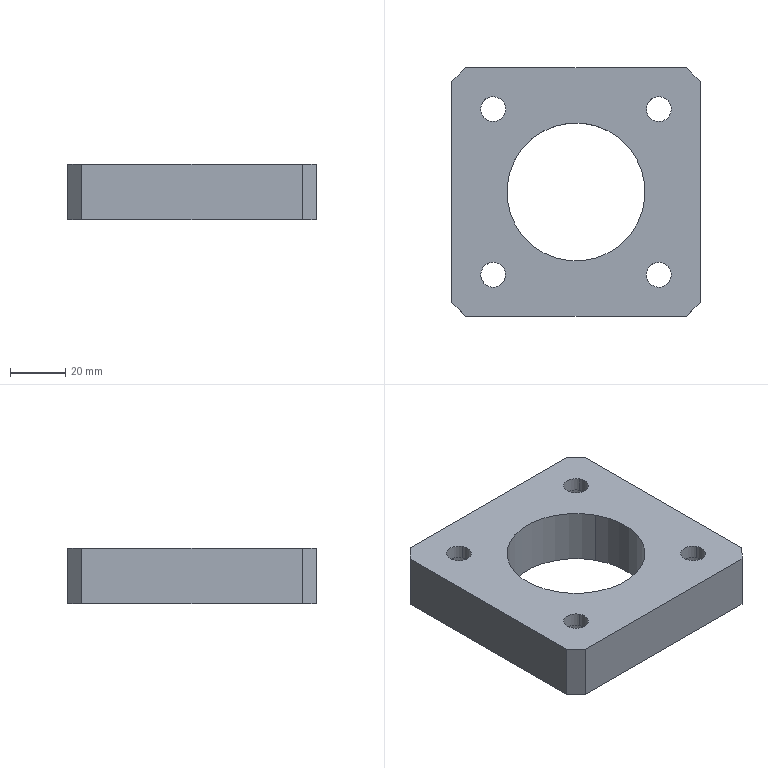Part | CATIA | 1 solid | 32 faces | box 90 x 90 x 20 mm | volume 109855 mm3 | cylinder 18 | plane 14 | commonest cylinder face diameters 9 x8 15 x8 50 x2
STEP:
#1=CARTESIAN_POINT('',(500.,-120.,-5.5));
#2=VERTEX_POINT('',#1);
#3=CARTESIAN_POINT('',(500.,-120.,14.5));
#4=VERTEX_POINT('',#3);
#5=CARTESIAN_POINT('',(500.,-120.,4.5));
#6=DIRECTION('',(0.,0.,-1.));
#7=VECTOR('',#6,1.);
#8=LINE('',#5,#7);
#9=EDGE_CURVE('',#2,#4,#8,.F.);
#10=ORIENTED_EDGE('',*,*,#9,.F.);
#11=CARTESIAN_POINT('',(495.,-125.,-5.5));
#12=VERTEX_POINT('',#11);
#13=CARTESIAN_POINT('',(497.5,-122.5,-5.5));
#14=DIRECTION('',(0.7071,0.7071,0.));
#15=VECTOR('',#14,1.);
#16=LINE('',#13,#15);
#17=EDGE_CURVE('',#2,#12,#16,.F.);
#18=ORIENTED_EDGE('',*,*,#17,.T.);
#19=CARTESIAN_POINT('',(495.,-125.,14.5));
#20=VERTEX_POINT('',#19);
#21=CARTESIAN_POINT('',(495.,-125.,4.5));
#22=DIRECTION('',(0.,0.,-1.));
#23=VECTOR('',#22,1.);
#24=LINE('',#21,#23);
#25=EDGE_CURVE('',#12,#20,#24,.F.);
#26=ORIENTED_EDGE('',*,*,#25,.T.);
#27=CARTESIAN_POINT('',(497.5,-122.5,14.5));
#28=DIRECTION('',(0.7071,0.7071,0.));
#29=VECTOR('',#28,1.);
#30=LINE('',#27,#29);
#31=EDGE_CURVE('',#20,#4,#30,.T.);
#32=ORIENTED_EDGE('',*,*,#31,.T.);
#33=EDGE_LOOP('',(#10,#18,#26,#32));
#34=FACE_OUTER_BOUND('',#33,.T.);
#35=CARTESIAN_POINT('',(495.,-125.,18.5));
#36=DIRECTION('',(0.7071,-0.7071,0.));
#37=DIRECTION('',(0.,0.,-1.));
#38=AXIS2_PLACEMENT_3D('',#35,#36,#37);
#39=PLANE('',#38);
#40=ADVANCED_FACE('',(#34),#39,.F.);
#41=CARTESIAN_POINT('',(495.,-205.,-5.5));
#42=VERTEX_POINT('',#41);
#43=CARTESIAN_POINT('',(495.,-205.,14.5));
#44=VERTEX_POINT('',#43);
#45=CARTESIAN_POINT('',(495.,-205.,4.5));
#46=DIRECTION('',(0.,0.,1.));
#47=VECTOR('',#46,1.);
#48=LINE('',#45,#47);
#49=EDGE_CURVE('',#42,#44,#48,.T.);
#50=ORIENTED_EDGE('',*,*,#49,.T.);
#51=CARTESIAN_POINT('',(495.,-165.,14.5));
#52=DIRECTION('',(0.,1.,0.));
#53=VECTOR('',#52,1.);
#54=LINE('',#51,#53);
#55=EDGE_CURVE('',#20,#44,#54,.F.);
#56=ORIENTED_EDGE('',*,*,#55,.F.);
#57=ORIENTED_EDGE('',*,*,#25,.F.);
#58=CARTESIAN_POINT('',(495.,-165.,-5.5));
#59=DIRECTION('',(0.,1.,0.));
#60=VECTOR('',#59,1.);
#61=LINE('',#58,#60);
#62=EDGE_CURVE('',#12,#42,#61,.F.);
#63=ORIENTED_EDGE('',*,*,#62,.T.);
#64=EDGE_LOOP('',(#50,#56,#57,#63));
#65=FACE_OUTER_BOUND('',#64,.T.);
#66=CARTESIAN_POINT('',(495.,-210.,-5.5));
#67=DIRECTION('',(1.,0.,0.));
#68=DIRECTION('',(0.,1.,0.));
#69=AXIS2_PLACEMENT_3D('',#66,#67,#68);
#70=PLANE('',#69);
#71=ADVANCED_FACE('',(#65),#70,.F.);
#72=ORIENTED_EDGE('',*,*,#49,.F.);
#73=CARTESIAN_POINT('',(500.,-210.,-5.5));
#74=VERTEX_POINT('',#73);
#75=CARTESIAN_POINT('',(497.5,-207.5,-5.5));
#76=DIRECTION('',(0.7071,-0.7071,0.));
#77=VECTOR('',#76,1.);
#78=LINE('',#75,#77);
#79=EDGE_CURVE('',#42,#74,#78,.T.);
#80=ORIENTED_EDGE('',*,*,#79,.T.);
#81=CARTESIAN_POINT('',(500.,-210.,14.5));
#82=VERTEX_POINT('',#81);
#83=CARTESIAN_POINT('',(500.,-210.,4.5));
#84=DIRECTION('',(0.,0.,1.));
#85=VECTOR('',#84,1.);
#86=LINE('',#83,#85);
#87=EDGE_CURVE('',#74,#82,#86,.T.);
#88=ORIENTED_EDGE('',*,*,#87,.T.);
#89=CARTESIAN_POINT('',(497.5,-207.5,14.5));
#90=DIRECTION('',(0.7071,-0.7071,0.));
#91=VECTOR('',#90,1.);
#92=LINE('',#89,#91);
#93=EDGE_CURVE('',#82,#44,#92,.F.);
#94=ORIENTED_EDGE('',*,*,#93,.T.);
#95=EDGE_LOOP('',(#72,#80,#88,#94));
#96=FACE_OUTER_BOUND('',#95,.T.);
#97=CARTESIAN_POINT('',(495.,-205.,-9.5));
#98=DIRECTION('',(0.7071,0.7071,0.));
#99=DIRECTION('',(0.,0.,1.));
#100=AXIS2_PLACEMENT_3D('',#97,#98,#99);
#101=PLANE('',#100);
#102=ADVANCED_FACE('',(#96),#101,.F.);
#103=CARTESIAN_POINT('',(580.,-210.,-5.5));
#104=VERTEX_POINT('',#103);
#105=CARTESIAN_POINT('',(580.,-210.,14.5));
#106=VERTEX_POINT('',#105);
#107=CARTESIAN_POINT('',(580.,-210.,4.5));
#108=DIRECTION('',(0.,0.,-1.));
#109=VECTOR('',#108,1.);
#110=LINE('',#107,#109);
#111=EDGE_CURVE('',#104,#106,#110,.F.);
#112=ORIENTED_EDGE('',*,*,#111,.T.);
#113=CARTESIAN_POINT('',(540.,-210.,14.5));
#114=DIRECTION('',(-1.,0.,0.));
#115=VECTOR('',#114,1.);
#116=LINE('',#113,#115);
#117=EDGE_CURVE('',#82,#106,#116,.F.);
#118=ORIENTED_EDGE('',*,*,#117,.F.);
#119=ORIENTED_EDGE('',*,*,#87,.F.);
#120=CARTESIAN_POINT('',(540.,-210.,-5.5));
#121=DIRECTION('',(-1.,0.,0.));
#122=VECTOR('',#121,1.);
#123=LINE('',#120,#122);
#124=EDGE_CURVE('',#74,#104,#123,.F.);
#125=ORIENTED_EDGE('',*,*,#124,.T.);
#126=EDGE_LOOP('',(#112,#118,#119,#125));
#127=FACE_OUTER_BOUND('',#126,.T.);
#128=CARTESIAN_POINT('',(585.,-210.,-5.5));
#129=DIRECTION('',(0.,1.,0.));
#130=DIRECTION('',(-1.,0.,0.));
#131=AXIS2_PLACEMENT_3D('',#128,#129,#130);
#132=PLANE('',#131);
#133=ADVANCED_FACE('',(#127),#132,.F.);
#134=ORIENTED_EDGE('',*,*,#111,.F.);
#135=CARTESIAN_POINT('',(585.,-205.,-5.5));
#136=VERTEX_POINT('',#135);
#137=CARTESIAN_POINT('',(582.5,-207.5,-5.5));
#138=DIRECTION('',(-0.7071,-0.7071,0.));
#139=VECTOR('',#138,1.);
#140=LINE('',#137,#139);
#141=EDGE_CURVE('',#104,#136,#140,.F.);
#142=ORIENTED_EDGE('',*,*,#141,.T.);
#143=CARTESIAN_POINT('',(585.,-205.,14.5));
#144=VERTEX_POINT('',#143);
#145=CARTESIAN_POINT('',(585.,-205.,4.5));
#146=DIRECTION('',(0.,0.,-1.));
#147=VECTOR('',#146,1.);
#148=LINE('',#145,#147);
#149=EDGE_CURVE('',#136,#144,#148,.F.);
#150=ORIENTED_EDGE('',*,*,#149,.T.);
#151=CARTESIAN_POINT('',(582.5,-207.5,14.5));
#152=DIRECTION('',(-0.7071,-0.7071,0.));
#153=VECTOR('',#152,1.);
#154=LINE('',#151,#153);
#155=EDGE_CURVE('',#144,#106,#154,.T.);
#156=ORIENTED_EDGE('',*,*,#155,.T.);
#157=EDGE_LOOP('',(#134,#142,#150,#156));
#158=FACE_OUTER_BOUND('',#157,.T.);
#159=CARTESIAN_POINT('',(585.,-205.,18.5));
#160=DIRECTION('',(-0.7071,0.7071,0.));
#161=DIRECTION('',(0.,0.,-1.));
#162=AXIS2_PLACEMENT_3D('',#159,#160,#161);
#163=PLANE('',#162);
#164=ADVANCED_FACE('',(#158),#163,.F.);
#165=CARTESIAN_POINT('',(580.,-120.,-5.5));
#166=VERTEX_POINT('',#165);
#167=CARTESIAN_POINT('',(580.,-120.,14.5));
#168=VERTEX_POINT('',#167);
#169=CARTESIAN_POINT('',(580.,-120.,4.5));
#170=DIRECTION('',(0.,0.,1.));
#171=VECTOR('',#170,1.);
#172=LINE('',#169,#171);
#173=EDGE_CURVE('',#166,#168,#172,.T.);
#174=ORIENTED_EDGE('',*,*,#173,.F.);
#175=CARTESIAN_POINT('',(540.,-120.,-5.5));
#176=DIRECTION('',(1.,0.,0.));
#177=VECTOR('',#176,1.);
#178=LINE('',#175,#177);
#179=EDGE_CURVE('',#166,#2,#178,.F.);
#180=ORIENTED_EDGE('',*,*,#179,.T.);
#181=ORIENTED_EDGE('',*,*,#9,.T.);
#182=CARTESIAN_POINT('',(540.,-120.,14.5));
#183=DIRECTION('',(1.,0.,0.));
#184=VECTOR('',#183,1.);
#185=LINE('',#182,#184);
#186=EDGE_CURVE('',#168,#4,#185,.F.);
#187=ORIENTED_EDGE('',*,*,#186,.F.);
#188=EDGE_LOOP('',(#174,#180,#181,#187));
#189=FACE_OUTER_BOUND('',#188,.T.);
#190=CARTESIAN_POINT('',(495.,-120.,-5.5));
#191=DIRECTION('',(0.,-1.,0.));
#192=DIRECTION('',(1.,0.,0.));
#193=AXIS2_PLACEMENT_3D('',#190,#191,#192);
#194=PLANE('',#193);
#195=ADVANCED_FACE('',(#189),#194,.F.);
#196=CARTESIAN_POINT('',(585.,-125.,-5.5));
#197=VERTEX_POINT('',#196);
#198=CARTESIAN_POINT('',(585.,-125.,14.5));
#199=VERTEX_POINT('',#198);
#200=CARTESIAN_POINT('',(585.,-125.,4.5));
#201=DIRECTION('',(0.,0.,1.));
#202=VECTOR('',#201,1.);
#203=LINE('',#200,#202);
#204=EDGE_CURVE('',#197,#199,#203,.T.);
#205=ORIENTED_EDGE('',*,*,#204,.T.);
#206=CARTESIAN_POINT('',(585.,-165.,14.5));
#207=DIRECTION('',(0.,-1.,0.));
#208=VECTOR('',#207,1.);
#209=LINE('',#206,#208);
#210=EDGE_CURVE('',#144,#199,#209,.F.);
#211=ORIENTED_EDGE('',*,*,#210,.F.);
#212=ORIENTED_EDGE('',*,*,#149,.F.);
#213=CARTESIAN_POINT('',(585.,-165.,-5.5));
#214=DIRECTION('',(0.,-1.,0.));
#215=VECTOR('',#214,1.);
#216=LINE('',#213,#215);
#217=EDGE_CURVE('',#136,#197,#216,.F.);
#218=ORIENTED_EDGE('',*,*,#217,.T.);
#219=EDGE_LOOP('',(#205,#211,#212,#218));
#220=FACE_OUTER_BOUND('',#219,.T.);
#221=CARTESIAN_POINT('',(585.,-120.,-5.5));
#222=DIRECTION('',(-1.,0.,0.));
#223=DIRECTION('',(0.,-1.,0.));
#224=AXIS2_PLACEMENT_3D('',#221,#222,#223);
#225=PLANE('',#224);
#226=ADVANCED_FACE('',(#220),#225,.F.);
#227=ORIENTED_EDGE('',*,*,#204,.F.);
#228=CARTESIAN_POINT('',(582.5,-122.5,-5.5));
#229=DIRECTION('',(-0.7071,0.7071,0.));
#230=VECTOR('',#229,1.);
#231=LINE('',#228,#230);
#232=EDGE_CURVE('',#197,#166,#231,.T.);
#233=ORIENTED_EDGE('',*,*,#232,.T.);
#234=ORIENTED_EDGE('',*,*,#173,.T.);
#235=CARTESIAN_POINT('',(582.5,-122.5,14.5));
#236=DIRECTION('',(-0.7071,0.7071,0.));
#237=VECTOR('',#236,1.);
#238=LINE('',#235,#237);
#239=EDGE_CURVE('',#168,#199,#238,.F.);
#240=ORIENTED_EDGE('',*,*,#239,.T.);
#241=EDGE_LOOP('',(#227,#233,#234,#240));
#242=FACE_OUTER_BOUND('',#241,.T.);
#243=CARTESIAN_POINT('',(585.,-125.,-9.5));
#244=DIRECTION('',(-0.7071,-0.7071,0.));
#245=DIRECTION('',(0.,0.,1.));
#246=AXIS2_PLACEMENT_3D('',#243,#244,#245);
#247=PLANE('',#246);
#248=ADVANCED_FACE('',(#242),#247,.F.);
#249=CARTESIAN_POINT('',(518.06,-176.986,14.5));
#250=VERTEX_POINT('',#249);
#251=CARTESIAN_POINT('',(561.94,-153.014,14.5));
#252=VERTEX_POINT('',#251);
#253=CARTESIAN_POINT('',(540.,-165.,14.5));
#254=DIRECTION('',(0.,0.,1.));
#255=AXIS2_PLACEMENT_3D('',#253,#254,$);
#256=CIRCLE('',#255,25.);
#257=EDGE_CURVE('',#250,#252,#256,.T.);
#258=ORIENTED_EDGE('',*,*,#257,.T.);
#259=CARTESIAN_POINT('',(561.94,-153.014,-5.5));
#260=VERTEX_POINT('',#259);
#261=CARTESIAN_POINT('',(561.94,-153.014,9.3));
#262=DIRECTION('',(0.,0.,1.));
#263=VECTOR('',#262,1.);
#264=LINE('',#261,#263);
#265=EDGE_CURVE('',#252,#260,#264,.F.);
#266=ORIENTED_EDGE('',*,*,#265,.T.);
#267=CARTESIAN_POINT('',(518.06,-176.986,-5.5));
#268=VERTEX_POINT('',#267);
#269=CARTESIAN_POINT('',(540.,-165.,-5.5));
#270=DIRECTION('',(0.,0.,1.));
#271=AXIS2_PLACEMENT_3D('',#269,#270,$);
#272=CIRCLE('',#271,25.);
#273=EDGE_CURVE('',#268,#260,#272,.T.);
#274=ORIENTED_EDGE('',*,*,#273,.F.);
#275=CARTESIAN_POINT('',(518.06,-176.986,9.3));
#276=DIRECTION('',(0.,0.,1.));
#277=VECTOR('',#276,1.);
#278=LINE('',#275,#277);
#279=EDGE_CURVE('',#250,#268,#278,.F.);
#280=ORIENTED_EDGE('',*,*,#279,.F.);
#281=EDGE_LOOP('',(#258,#266,#274,#280));
#282=FACE_OUTER_BOUND('',#281,.T.);
#283=CARTESIAN_POINT('',(540.,-165.,-5.4));
#284=DIRECTION('',(0.,0.,1.));
#285=DIRECTION('',(0.8776,0.4794,0.));
#286=AXIS2_PLACEMENT_3D('',#283,#284,#285);
#287=CYLINDRICAL_SURFACE('',#286,25.);
#288=ADVANCED_FACE('',(#282),#287,.F.);
#289=CARTESIAN_POINT('',(540.,-165.,14.5));
#290=DIRECTION('',(0.,0.,1.));
#291=AXIS2_PLACEMENT_3D('',#289,#290,$);
#292=CIRCLE('',#291,25.);
#293=EDGE_CURVE('',#252,#250,#292,.T.);
#294=ORIENTED_EDGE('',*,*,#293,.T.);
#295=ORIENTED_EDGE('',*,*,#279,.T.);
#296=CARTESIAN_POINT('',(540.,-165.,-5.5));
#297=DIRECTION('',(0.,0.,1.));
#298=AXIS2_PLACEMENT_3D('',#296,#297,$);
#299=CIRCLE('',#298,25.);
#300=EDGE_CURVE('',#260,#268,#299,.T.);
#301=ORIENTED_EDGE('',*,*,#300,.F.);
#302=ORIENTED_EDGE('',*,*,#265,.F.);
#303=EDGE_LOOP('',(#294,#295,#301,#302));
#304=FACE_OUTER_BOUND('',#303,.T.);
#305=ADVANCED_FACE('',(#304),#287,.F.);
#306=ORIENTED_EDGE('',*,*,#232,.F.);
#307=ORIENTED_EDGE('',*,*,#217,.F.);
#308=ORIENTED_EDGE('',*,*,#141,.F.);
#309=ORIENTED_EDGE('',*,*,#124,.F.);
#310=ORIENTED_EDGE('',*,*,#79,.F.);
#311=ORIENTED_EDGE('',*,*,#62,.F.);
#312=ORIENTED_EDGE('',*,*,#17,.F.);
#313=ORIENTED_EDGE('',*,*,#179,.F.);
#314=EDGE_LOOP('',(#306,#307,#308,#309,#310,#311,#312,#313));
#315=FACE_OUTER_BOUND('',#314,.T.);
#316=ORIENTED_EDGE('',*,*,#300,.T.);
#317=ORIENTED_EDGE('',*,*,#273,.T.);
#318=EDGE_LOOP('',(#316,#317));
#319=FACE_BOUND('',#318,.T.);
#320=CARTESIAN_POINT('',(576.582,-191.404,-5.5));
#321=VERTEX_POINT('',#320);
#322=CARTESIAN_POINT('',(563.418,-198.596,-5.5));
#323=VERTEX_POINT('',#322);
#324=CARTESIAN_POINT('',(570.,-195.,-5.5));
#325=DIRECTION('',(0.,0.,1.));
#326=AXIS2_PLACEMENT_3D('',#324,#325,$);
#327=CIRCLE('',#326,7.5);
#328=EDGE_CURVE('',#321,#323,#327,.T.);
#329=ORIENTED_EDGE('',*,*,#328,.T.);
#330=CARTESIAN_POINT('',(570.,-195.,-5.5));
#331=DIRECTION('',(0.,0.,1.));
#332=AXIS2_PLACEMENT_3D('',#330,#331,$);
#333=CIRCLE('',#332,7.5);
#334=EDGE_CURVE('',#323,#321,#333,.T.);
#335=ORIENTED_EDGE('',*,*,#334,.T.);
#336=EDGE_LOOP('',(#329,#335));
#337=FACE_BOUND('',#336,.T.);
#338=CARTESIAN_POINT('',(516.582,-191.404,-5.5));
#339=VERTEX_POINT('',#338);
#340=CARTESIAN_POINT('',(503.418,-198.596,-5.5));
#341=VERTEX_POINT('',#340);
#342=CARTESIAN_POINT('',(510.,-195.,-5.5));
#343=DIRECTION('',(0.,0.,1.));
#344=AXIS2_PLACEMENT_3D('',#342,#343,$);
#345=CIRCLE('',#344,7.5);
#346=EDGE_CURVE('',#339,#341,#345,.T.);
#347=ORIENTED_EDGE('',*,*,#346,.T.);
#348=CARTESIAN_POINT('',(510.,-195.,-5.5));
#349=DIRECTION('',(0.,0.,1.));
#350=AXIS2_PLACEMENT_3D('',#348,#349,$);
#351=CIRCLE('',#350,7.5);
#352=EDGE_CURVE('',#341,#339,#351,.T.);
#353=ORIENTED_EDGE('',*,*,#352,.T.);
#354=EDGE_LOOP('',(#347,#353));
#355=FACE_BOUND('',#354,.T.);
#356=CARTESIAN_POINT('',(576.582,-131.404,-5.5));
#357=VERTEX_POINT('',#356);
#358=CARTESIAN_POINT('',(563.418,-138.596,-5.5));
#359=VERTEX_POINT('',#358);
#360=CARTESIAN_POINT('',(570.,-135.,-5.5));
#361=DIRECTION('',(0.,0.,1.));
#362=AXIS2_PLACEMENT_3D('',#360,#361,$);
#363=CIRCLE('',#362,7.5);
#364=EDGE_CURVE('',#357,#359,#363,.T.);
#365=ORIENTED_EDGE('',*,*,#364,.T.);
#366=CARTESIAN_POINT('',(570.,-135.,-5.5));
#367=DIRECTION('',(0.,0.,1.));
#368=AXIS2_PLACEMENT_3D('',#366,#367,$);
#369=CIRCLE('',#368,7.5);
#370=EDGE_CURVE('',#359,#357,#369,.T.);
#371=ORIENTED_EDGE('',*,*,#370,.T.);
#372=EDGE_LOOP('',(#365,#371));
#373=FACE_BOUND('',#372,.T.);
#374=CARTESIAN_POINT('',(516.582,-131.404,-5.5));
#375=VERTEX_POINT('',#374);
#376=CARTESIAN_POINT('',(503.418,-138.596,-5.5));
#377=VERTEX_POINT('',#376);
#378=CARTESIAN_POINT('',(510.,-135.,-5.5));
#379=DIRECTION('',(0.,0.,1.));
#380=AXIS2_PLACEMENT_3D('',#378,#379,$);
#381=CIRCLE('',#380,7.5);
#382=EDGE_CURVE('',#375,#377,#381,.T.);
#383=ORIENTED_EDGE('',*,*,#382,.T.);
#384=CARTESIAN_POINT('',(510.,-135.,-5.5));
#385=DIRECTION('',(0.,0.,1.));
#386=AXIS2_PLACEMENT_3D('',#384,#385,$);
#387=CIRCLE('',#386,7.5);
#388=EDGE_CURVE('',#377,#375,#387,.T.);
#389=ORIENTED_EDGE('',*,*,#388,.T.);
#390=EDGE_LOOP('',(#383,#389));
#391=FACE_BOUND('',#390,.T.);
#392=CARTESIAN_POINT('',(0.,0.,-5.5));
#393=DIRECTION('',(0.,0.,1.));
#394=DIRECTION('',(1.,0.,0.));
#395=AXIS2_PLACEMENT_3D('',#392,#393,#394);
#396=PLANE('',#395);
#397=ADVANCED_FACE('',(#315,#319,#337,#355,#373,#391),#396,.F.);
#398=ORIENTED_EDGE('',*,*,#186,.T.);
#399=ORIENTED_EDGE('',*,*,#31,.F.);
#400=ORIENTED_EDGE('',*,*,#55,.T.);
#401=ORIENTED_EDGE('',*,*,#93,.F.);
#402=ORIENTED_EDGE('',*,*,#117,.T.);
#403=ORIENTED_EDGE('',*,*,#155,.F.);
#404=ORIENTED_EDGE('',*,*,#210,.T.);
#405=ORIENTED_EDGE('',*,*,#239,.F.);
#406=EDGE_LOOP('',(#398,#399,#400,#401,#402,#403,#404,#405));
#407=FACE_OUTER_BOUND('',#406,.T.);
#408=ORIENTED_EDGE('',*,*,#293,.F.);
#409=ORIENTED_EDGE('',*,*,#257,.F.);
#410=EDGE_LOOP('',(#408,#409));
#411=FACE_BOUND('',#410,.T.);
#412=CARTESIAN_POINT('',(566.051,-197.157,14.5));
#413=VERTEX_POINT('',#412);
#414=CARTESIAN_POINT('',(573.949,-192.843,14.5));
#415=VERTEX_POINT('',#414);
#416=CARTESIAN_POINT('',(570.,-195.,14.5));
#417=DIRECTION('',(0.,0.,1.));
#418=AXIS2_PLACEMENT_3D('',#416,#417,$);
#419=CIRCLE('',#418,4.5);
#420=EDGE_CURVE('',#413,#415,#419,.T.);
#421=ORIENTED_EDGE('',*,*,#420,.F.);
#422=CARTESIAN_POINT('',(570.,-195.,14.5));
#423=DIRECTION('',(0.,0.,1.));
#424=AXIS2_PLACEMENT_3D('',#422,#423,$);
#425=CIRCLE('',#424,4.5);
#426=EDGE_CURVE('',#415,#413,#425,.T.);
#427=ORIENTED_EDGE('',*,*,#426,.F.);
#428=EDGE_LOOP('',(#421,#427));
#429=FACE_BOUND('',#428,.T.);
#430=CARTESIAN_POINT('',(506.051,-197.157,14.5));
#431=VERTEX_POINT('',#430);
#432=CARTESIAN_POINT('',(513.949,-192.843,14.5));
#433=VERTEX_POINT('',#432);
#434=CARTESIAN_POINT('',(510.,-195.,14.5));
#435=DIRECTION('',(0.,0.,1.));
#436=AXIS2_PLACEMENT_3D('',#434,#435,$);
#437=CIRCLE('',#436,4.5);
#438=EDGE_CURVE('',#431,#433,#437,.T.);
#439=ORIENTED_EDGE('',*,*,#438,.F.);
#440=CARTESIAN_POINT('',(510.,-195.,14.5));
#441=DIRECTION('',(0.,0.,1.));
#442=AXIS2_PLACEMENT_3D('',#440,#441,$);
#443=CIRCLE('',#442,4.5);
#444=EDGE_CURVE('',#433,#431,#443,.T.);
#445=ORIENTED_EDGE('',*,*,#444,.F.);
#446=EDGE_LOOP('',(#439,#445));
#447=FACE_BOUND('',#446,.T.);
#448=CARTESIAN_POINT('',(566.051,-137.157,14.5));
#449=VERTEX_POINT('',#448);
#450=CARTESIAN_POINT('',(573.949,-132.843,14.5));
#451=VERTEX_POINT('',#450);
#452=CARTESIAN_POINT('',(570.,-135.,14.5));
#453=DIRECTION('',(0.,0.,1.));
#454=AXIS2_PLACEMENT_3D('',#452,#453,$);
#455=CIRCLE('',#454,4.5);
#456=EDGE_CURVE('',#449,#451,#455,.T.);
#457=ORIENTED_EDGE('',*,*,#456,.F.);
#458=CARTESIAN_POINT('',(570.,-135.,14.5));
#459=DIRECTION('',(0.,0.,1.));
#460=AXIS2_PLACEMENT_3D('',#458,#459,$);
#461=CIRCLE('',#460,4.5);
#462=EDGE_CURVE('',#451,#449,#461,.T.);
#463=ORIENTED_EDGE('',*,*,#462,.F.);
#464=EDGE_LOOP('',(#457,#463));
#465=FACE_BOUND('',#464,.T.);
#466=CARTESIAN_POINT('',(506.051,-137.157,14.5));
#467=VERTEX_POINT('',#466);
#468=CARTESIAN_POINT('',(513.949,-132.843,14.5));
#469=VERTEX_POINT('',#468);
#470=CARTESIAN_POINT('',(510.,-135.,14.5));
#471=DIRECTION('',(0.,0.,1.));
#472=AXIS2_PLACEMENT_3D('',#470,#471,$);
#473=CIRCLE('',#472,4.5);
#474=EDGE_CURVE('',#467,#469,#473,.T.);
#475=ORIENTED_EDGE('',*,*,#474,.F.);
#476=CARTESIAN_POINT('',(510.,-135.,14.5));
#477=DIRECTION('',(0.,0.,1.));
#478=AXIS2_PLACEMENT_3D('',#476,#477,$);
#479=CIRCLE('',#478,4.5);
#480=EDGE_CURVE('',#469,#467,#479,.T.);
#481=ORIENTED_EDGE('',*,*,#480,.F.);
#482=EDGE_LOOP('',(#475,#481));
#483=FACE_BOUND('',#482,.T.);
#484=CARTESIAN_POINT('',(0.,0.,14.5));
#485=DIRECTION('',(0.,0.,1.));
#486=DIRECTION('',(1.,0.,0.));
#487=AXIS2_PLACEMENT_3D('',#484,#485,#486);
#488=PLANE('',#487);
#489=ADVANCED_FACE('',(#407,#411,#429,#447,#465,#483),#488,.T.);
#490=CARTESIAN_POINT('',(576.582,-131.404,9.5));
#491=VERTEX_POINT('',#490);
#492=CARTESIAN_POINT('',(563.418,-138.596,9.5));
#493=VERTEX_POINT('',#492);
#494=CARTESIAN_POINT('',(570.,-135.,9.5));
#495=DIRECTION('',(0.,0.,1.));
#496=AXIS2_PLACEMENT_3D('',#494,#495,$);
#497=CIRCLE('',#496,7.5);
#498=EDGE_CURVE('',#491,#493,#497,.T.);
#499=ORIENTED_EDGE('',*,*,#498,.F.);
#500=CARTESIAN_POINT('',(570.,-135.,9.5));
#501=DIRECTION('',(0.,0.,1.));
#502=AXIS2_PLACEMENT_3D('',#500,#501,$);
#503=CIRCLE('',#502,7.5);
#504=EDGE_CURVE('',#493,#491,#503,.T.);
#505=ORIENTED_EDGE('',*,*,#504,.F.);
#506=EDGE_LOOP('',(#499,#505));
#507=FACE_OUTER_BOUND('',#506,.T.);
#508=CARTESIAN_POINT('',(566.051,-137.157,9.5));
#509=VERTEX_POINT('',#508);
#510=CARTESIAN_POINT('',(573.949,-132.843,9.5));
#511=VERTEX_POINT('',#510);
#512=CARTESIAN_POINT('',(570.,-135.,9.5));
#513=DIRECTION('',(0.,0.,1.));
#514=AXIS2_PLACEMENT_3D('',#512,#513,$);
#515=CIRCLE('',#514,4.5);
#516=EDGE_CURVE('',#509,#511,#515,.T.);
#517=ORIENTED_EDGE('',*,*,#516,.T.);
#518=CARTESIAN_POINT('',(570.,-135.,9.5));
#519=DIRECTION('',(0.,0.,1.));
#520=AXIS2_PLACEMENT_3D('',#518,#519,$);
#521=CIRCLE('',#520,4.5);
#522=EDGE_CURVE('',#511,#509,#521,.T.);
#523=ORIENTED_EDGE('',*,*,#522,.T.);
#524=EDGE_LOOP('',(#517,#523));
#525=FACE_BOUND('',#524,.T.);
#526=CARTESIAN_POINT('',(574.5,-195.,9.5));
#527=DIRECTION('',(0.,0.,1.));
#528=DIRECTION('',(1.,0.,0.));
#529=AXIS2_PLACEMENT_3D('',#526,#527,#528);
#530=PLANE('',#529);
#531=ADVANCED_FACE('',(#507,#525),#530,.F.);
#532=ORIENTED_EDGE('',*,*,#370,.F.);
#533=CARTESIAN_POINT('',(563.418,-138.596,1.8));
#534=DIRECTION('',(0.,0.,1.));
#535=VECTOR('',#534,1.);
#536=LINE('',#533,#535);
#537=EDGE_CURVE('',#493,#359,#536,.F.);
#538=ORIENTED_EDGE('',*,*,#537,.F.);
#539=ORIENTED_EDGE('',*,*,#504,.T.);
#540=CARTESIAN_POINT('',(576.582,-131.404,1.8));
#541=DIRECTION('',(0.,0.,1.));
#542=VECTOR('',#541,1.);
#543=LINE('',#540,#542);
#544=EDGE_CURVE('',#491,#357,#543,.F.);
#545=ORIENTED_EDGE('',*,*,#544,.T.);
#546=EDGE_LOOP('',(#532,#538,#539,#545));
#547=FACE_OUTER_BOUND('',#546,.T.);
#548=CARTESIAN_POINT('',(570.,-135.,-5.4));
#549=DIRECTION('',(0.,0.,1.));
#550=DIRECTION('',(0.8776,0.4794,0.));
#551=AXIS2_PLACEMENT_3D('',#548,#549,#550);
#552=CYLINDRICAL_SURFACE('',#551,7.5);
#553=ADVANCED_FACE('',(#547),#552,.F.);
#554=ORIENTED_EDGE('',*,*,#364,.F.);
#555=ORIENTED_EDGE('',*,*,#544,.F.);
#556=ORIENTED_EDGE('',*,*,#498,.T.);
#557=ORIENTED_EDGE('',*,*,#537,.T.);
#558=EDGE_LOOP('',(#554,#555,#556,#557));
#559=FACE_OUTER_BOUND('',#558,.T.);
#560=ADVANCED_FACE('',(#559),#552,.F.);
#561=ORIENTED_EDGE('',*,*,#462,.T.);
#562=CARTESIAN_POINT('',(566.051,-137.157,12.2));
#563=DIRECTION('',(0.,0.,1.));
#564=VECTOR('',#563,1.);
#565=LINE('',#562,#564);
#566=EDGE_CURVE('',#449,#509,#565,.F.);
#567=ORIENTED_EDGE('',*,*,#566,.T.);
#568=ORIENTED_EDGE('',*,*,#522,.F.);
#569=CARTESIAN_POINT('',(573.949,-132.843,12.2));
#570=DIRECTION('',(0.,0.,1.));
#571=VECTOR('',#570,1.);
#572=LINE('',#569,#571);
#573=EDGE_CURVE('',#451,#511,#572,.F.);
#574=ORIENTED_EDGE('',*,*,#573,.F.);
#575=EDGE_LOOP('',(#561,#567,#568,#574));
#576=FACE_OUTER_BOUND('',#575,.T.);
#577=CARTESIAN_POINT('',(570.,-135.,-5.4));
#578=DIRECTION('',(0.,0.,1.));
#579=DIRECTION('',(0.8776,0.4794,0.));
#580=AXIS2_PLACEMENT_3D('',#577,#578,#579);
#581=CYLINDRICAL_SURFACE('',#580,4.5);
#582=ADVANCED_FACE('',(#576),#581,.F.);
#583=ORIENTED_EDGE('',*,*,#456,.T.);
#584=ORIENTED_EDGE('',*,*,#573,.T.);
#585=ORIENTED_EDGE('',*,*,#516,.F.);
#586=ORIENTED_EDGE('',*,*,#566,.F.);
#587=EDGE_LOOP('',(#583,#584,#585,#586));
#588=FACE_OUTER_BOUND('',#587,.T.);
#589=ADVANCED_FACE('',(#588),#581,.F.);
#590=CARTESIAN_POINT('',(516.582,-191.404,9.5));
#591=VERTEX_POINT('',#590);
#592=CARTESIAN_POINT('',(503.418,-198.596,9.5));
#593=VERTEX_POINT('',#592);
#594=CARTESIAN_POINT('',(510.,-195.,9.5));
#595=DIRECTION('',(0.,0.,1.));
#596=AXIS2_PLACEMENT_3D('',#594,#595,$);
#597=CIRCLE('',#596,7.5);
#598=EDGE_CURVE('',#591,#593,#597,.T.);
#599=ORIENTED_EDGE('',*,*,#598,.F.);
#600=CARTESIAN_POINT('',(510.,-195.,9.5));
#601=DIRECTION('',(0.,0.,1.));
#602=AXIS2_PLACEMENT_3D('',#600,#601,$);
#603=CIRCLE('',#602,7.5);
#604=EDGE_CURVE('',#593,#591,#603,.T.);
#605=ORIENTED_EDGE('',*,*,#604,.F.);
#606=EDGE_LOOP('',(#599,#605));
#607=FACE_OUTER_BOUND('',#606,.T.);
#608=CARTESIAN_POINT('',(506.051,-197.157,9.5));
#609=VERTEX_POINT('',#608);
#610=CARTESIAN_POINT('',(513.949,-192.843,9.5));
#611=VERTEX_POINT('',#610);
#612=CARTESIAN_POINT('',(510.,-195.,9.5));
#613=DIRECTION('',(0.,0.,1.));
#614=AXIS2_PLACEMENT_3D('',#612,#613,$);
#615=CIRCLE('',#614,4.5);
#616=EDGE_CURVE('',#609,#611,#615,.T.);
#617=ORIENTED_EDGE('',*,*,#616,.T.);
#618=CARTESIAN_POINT('',(510.,-195.,9.5));
#619=DIRECTION('',(0.,0.,1.));
#620=AXIS2_PLACEMENT_3D('',#618,#619,$);
#621=CIRCLE('',#620,4.5);
#622=EDGE_CURVE('',#611,#609,#621,.T.);
#623=ORIENTED_EDGE('',*,*,#622,.T.);
#624=EDGE_LOOP('',(#617,#623));
#625=FACE_BOUND('',#624,.T.);
#626=ADVANCED_FACE('',(#607,#625),#530,.F.);
#627=ORIENTED_EDGE('',*,*,#352,.F.);
#628=CARTESIAN_POINT('',(503.418,-198.596,1.8));
#629=DIRECTION('',(0.,0.,1.));
#630=VECTOR('',#629,1.);
#631=LINE('',#628,#630);
#632=EDGE_CURVE('',#593,#341,#631,.F.);
#633=ORIENTED_EDGE('',*,*,#632,.F.);
#634=ORIENTED_EDGE('',*,*,#604,.T.);
#635=CARTESIAN_POINT('',(516.582,-191.404,1.8));
#636=DIRECTION('',(0.,0.,1.));
#637=VECTOR('',#636,1.);
#638=LINE('',#635,#637);
#639=EDGE_CURVE('',#591,#339,#638,.F.);
#640=ORIENTED_EDGE('',*,*,#639,.T.);
#641=EDGE_LOOP('',(#627,#633,#634,#640));
#642=FACE_OUTER_BOUND('',#641,.T.);
#643=CARTESIAN_POINT('',(510.,-195.,-5.4));
#644=DIRECTION('',(0.,0.,1.));
#645=DIRECTION('',(0.8776,0.4794,0.));
#646=AXIS2_PLACEMENT_3D('',#643,#644,#645);
#647=CYLINDRICAL_SURFACE('',#646,7.5);
#648=ADVANCED_FACE('',(#642),#647,.F.);
#649=ORIENTED_EDGE('',*,*,#346,.F.);
#650=ORIENTED_EDGE('',*,*,#639,.F.);
#651=ORIENTED_EDGE('',*,*,#598,.T.);
#652=ORIENTED_EDGE('',*,*,#632,.T.);
#653=EDGE_LOOP('',(#649,#650,#651,#652));
#654=FACE_OUTER_BOUND('',#653,.T.);
#655=ADVANCED_FACE('',(#654),#647,.F.);
#656=ORIENTED_EDGE('',*,*,#444,.T.);
#657=CARTESIAN_POINT('',(506.051,-197.157,12.2));
#658=DIRECTION('',(0.,0.,1.));
#659=VECTOR('',#658,1.);
#660=LINE('',#657,#659);
#661=EDGE_CURVE('',#431,#609,#660,.F.);
#662=ORIENTED_EDGE('',*,*,#661,.T.);
#663=ORIENTED_EDGE('',*,*,#622,.F.);
#664=CARTESIAN_POINT('',(513.949,-192.843,12.2));
#665=DIRECTION('',(0.,0.,1.));
#666=VECTOR('',#665,1.);
#667=LINE('',#664,#666);
#668=EDGE_CURVE('',#433,#611,#667,.F.);
#669=ORIENTED_EDGE('',*,*,#668,.F.);
#670=EDGE_LOOP('',(#656,#662,#663,#669));
#671=FACE_OUTER_BOUND('',#670,.T.);
#672=CARTESIAN_POINT('',(510.,-195.,-5.4));
#673=DIRECTION('',(0.,0.,1.));
#674=DIRECTION('',(0.8776,0.4794,0.));
#675=AXIS2_PLACEMENT_3D('',#672,#673,#674);
#676=CYLINDRICAL_SURFACE('',#675,4.5);
#677=ADVANCED_FACE('',(#671),#676,.F.);
#678=ORIENTED_EDGE('',*,*,#438,.T.);
#679=ORIENTED_EDGE('',*,*,#668,.T.);
#680=ORIENTED_EDGE('',*,*,#616,.F.);
#681=ORIENTED_EDGE('',*,*,#661,.F.);
#682=EDGE_LOOP('',(#678,#679,#680,#681));
#683=FACE_OUTER_BOUND('',#682,.T.);
#684=ADVANCED_FACE('',(#683),#676,.F.);
#685=CARTESIAN_POINT('',(516.582,-131.404,9.5));
#686=VERTEX_POINT('',#685);
#687=CARTESIAN_POINT('',(503.418,-138.596,9.5));
#688=VERTEX_POINT('',#687);
#689=CARTESIAN_POINT('',(510.,-135.,9.5));
#690=DIRECTION('',(0.,0.,1.));
#691=AXIS2_PLACEMENT_3D('',#689,#690,$);
#692=CIRCLE('',#691,7.5);
#693=EDGE_CURVE('',#686,#688,#692,.T.);
#694=ORIENTED_EDGE('',*,*,#693,.F.);
#695=CARTESIAN_POINT('',(510.,-135.,9.5));
#696=DIRECTION('',(0.,0.,1.));
#697=AXIS2_PLACEMENT_3D('',#695,#696,$);
#698=CIRCLE('',#697,7.5);
#699=EDGE_CURVE('',#688,#686,#698,.T.);
#700=ORIENTED_EDGE('',*,*,#699,.F.);
#701=EDGE_LOOP('',(#694,#700));
#702=FACE_OUTER_BOUND('',#701,.T.);
#703=CARTESIAN_POINT('',(506.051,-137.157,9.5));
#704=VERTEX_POINT('',#703);
#705=CARTESIAN_POINT('',(513.949,-132.843,9.5));
#706=VERTEX_POINT('',#705);
#707=CARTESIAN_POINT('',(510.,-135.,9.5));
#708=DIRECTION('',(0.,0.,1.));
#709=AXIS2_PLACEMENT_3D('',#707,#708,$);
#710=CIRCLE('',#709,4.5);
#711=EDGE_CURVE('',#704,#706,#710,.T.);
#712=ORIENTED_EDGE('',*,*,#711,.T.);
#713=CARTESIAN_POINT('',(510.,-135.,9.5));
#714=DIRECTION('',(0.,0.,1.));
#715=AXIS2_PLACEMENT_3D('',#713,#714,$);
#716=CIRCLE('',#715,4.5);
#717=EDGE_CURVE('',#706,#704,#716,.T.);
#718=ORIENTED_EDGE('',*,*,#717,.T.);
#719=EDGE_LOOP('',(#712,#718));
#720=FACE_BOUND('',#719,.T.);
#721=ADVANCED_FACE('',(#702,#720),#530,.F.);
#722=ORIENTED_EDGE('',*,*,#388,.F.);
#723=CARTESIAN_POINT('',(503.418,-138.596,1.8));
#724=DIRECTION('',(0.,0.,1.));
#725=VECTOR('',#724,1.);
#726=LINE('',#723,#725);
#727=EDGE_CURVE('',#688,#377,#726,.F.);
#728=ORIENTED_EDGE('',*,*,#727,.F.);
#729=ORIENTED_EDGE('',*,*,#699,.T.);
#730=CARTESIAN_POINT('',(516.582,-131.404,1.8));
#731=DIRECTION('',(0.,0.,1.));
#732=VECTOR('',#731,1.);
#733=LINE('',#730,#732);
#734=EDGE_CURVE('',#686,#375,#733,.F.);
#735=ORIENTED_EDGE('',*,*,#734,.T.);
#736=EDGE_LOOP('',(#722,#728,#729,#735));
#737=FACE_OUTER_BOUND('',#736,.T.);
#738=CARTESIAN_POINT('',(510.,-135.,-5.4));
#739=DIRECTION('',(0.,0.,1.));
#740=DIRECTION('',(0.8776,0.4794,0.));
#741=AXIS2_PLACEMENT_3D('',#738,#739,#740);
#742=CYLINDRICAL_SURFACE('',#741,7.5);
#743=ADVANCED_FACE('',(#737),#742,.F.);
#744=ORIENTED_EDGE('',*,*,#382,.F.);
#745=ORIENTED_EDGE('',*,*,#734,.F.);
#746=ORIENTED_EDGE('',*,*,#693,.T.);
#747=ORIENTED_EDGE('',*,*,#727,.T.);
#748=EDGE_LOOP('',(#744,#745,#746,#747));
#749=FACE_OUTER_BOUND('',#748,.T.);
#750=ADVANCED_FACE('',(#749),#742,.F.);
#751=ORIENTED_EDGE('',*,*,#480,.T.);
#752=CARTESIAN_POINT('',(506.051,-137.157,12.2));
#753=DIRECTION('',(0.,0.,1.));
#754=VECTOR('',#753,1.);
#755=LINE('',#752,#754);
#756=EDGE_CURVE('',#467,#704,#755,.F.);
#757=ORIENTED_EDGE('',*,*,#756,.T.);
#758=ORIENTED_EDGE('',*,*,#717,.F.);
#759=CARTESIAN_POINT('',(513.949,-132.843,12.2));
#760=DIRECTION('',(0.,0.,1.));
#761=VECTOR('',#760,1.);
#762=LINE('',#759,#761);
#763=EDGE_CURVE('',#469,#706,#762,.F.);
#764=ORIENTED_EDGE('',*,*,#763,.F.);
#765=EDGE_LOOP('',(#751,#757,#758,#764));
#766=FACE_OUTER_BOUND('',#765,.T.);
#767=CARTESIAN_POINT('',(510.,-135.,-5.4));
#768=DIRECTION('',(0.,0.,1.));
#769=DIRECTION('',(0.8776,0.4794,0.));
#770=AXIS2_PLACEMENT_3D('',#767,#768,#769);
#771=CYLINDRICAL_SURFACE('',#770,4.5);
#772=ADVANCED_FACE('',(#766),#771,.F.);
#773=ORIENTED_EDGE('',*,*,#474,.T.);
#774=ORIENTED_EDGE('',*,*,#763,.T.);
#775=ORIENTED_EDGE('',*,*,#711,.F.);
#776=ORIENTED_EDGE('',*,*,#756,.F.);
#777=EDGE_LOOP('',(#773,#774,#775,#776));
#778=FACE_OUTER_BOUND('',#777,.T.);
#779=ADVANCED_FACE('',(#778),#771,.F.);
#780=CARTESIAN_POINT('',(576.582,-191.404,9.5));
#781=VERTEX_POINT('',#780);
#782=CARTESIAN_POINT('',(563.418,-198.596,9.5));
#783=VERTEX_POINT('',#782);
#784=CARTESIAN_POINT('',(570.,-195.,9.5));
#785=DIRECTION('',(0.,0.,1.));
#786=AXIS2_PLACEMENT_3D('',#784,#785,$);
#787=CIRCLE('',#786,7.5);
#788=EDGE_CURVE('',#781,#783,#787,.T.);
#789=ORIENTED_EDGE('',*,*,#788,.F.);
#790=CARTESIAN_POINT('',(570.,-195.,9.5));
#791=DIRECTION('',(0.,0.,1.));
#792=AXIS2_PLACEMENT_3D('',#790,#791,$);
#793=CIRCLE('',#792,7.5);
#794=EDGE_CURVE('',#783,#781,#793,.T.);
#795=ORIENTED_EDGE('',*,*,#794,.F.);
#796=EDGE_LOOP('',(#789,#795));
#797=FACE_OUTER_BOUND('',#796,.T.);
#798=CARTESIAN_POINT('',(566.051,-197.157,9.5));
#799=VERTEX_POINT('',#798);
#800=CARTESIAN_POINT('',(573.949,-192.843,9.5));
#801=VERTEX_POINT('',#800);
#802=CARTESIAN_POINT('',(570.,-195.,9.5));
#803=DIRECTION('',(0.,0.,1.));
#804=AXIS2_PLACEMENT_3D('',#802,#803,$);
#805=CIRCLE('',#804,4.5);
#806=EDGE_CURVE('',#799,#801,#805,.T.);
#807=ORIENTED_EDGE('',*,*,#806,.T.);
#808=CARTESIAN_POINT('',(570.,-195.,9.5));
#809=DIRECTION('',(0.,0.,1.));
#810=AXIS2_PLACEMENT_3D('',#808,#809,$);
#811=CIRCLE('',#810,4.5);
#812=EDGE_CURVE('',#801,#799,#811,.T.);
#813=ORIENTED_EDGE('',*,*,#812,.T.);
#814=EDGE_LOOP('',(#807,#813));
#815=FACE_BOUND('',#814,.T.);
#816=ADVANCED_FACE('',(#797,#815),#530,.F.);
#817=ORIENTED_EDGE('',*,*,#334,.F.);
#818=CARTESIAN_POINT('',(563.418,-198.596,1.8));
#819=DIRECTION('',(0.,0.,1.));
#820=VECTOR('',#819,1.);
#821=LINE('',#818,#820);
#822=EDGE_CURVE('',#783,#323,#821,.F.);
#823=ORIENTED_EDGE('',*,*,#822,.F.);
#824=ORIENTED_EDGE('',*,*,#794,.T.);
#825=CARTESIAN_POINT('',(576.582,-191.404,1.8));
#826=DIRECTION('',(0.,0.,1.));
#827=VECTOR('',#826,1.);
#828=LINE('',#825,#827);
#829=EDGE_CURVE('',#781,#321,#828,.F.);
#830=ORIENTED_EDGE('',*,*,#829,.T.);
#831=EDGE_LOOP('',(#817,#823,#824,#830));
#832=FACE_OUTER_BOUND('',#831,.T.);
#833=CARTESIAN_POINT('',(570.,-195.,-5.4));
#834=DIRECTION('',(0.,0.,1.));
#835=DIRECTION('',(0.8776,0.4794,0.));
#836=AXIS2_PLACEMENT_3D('',#833,#834,#835);
#837=CYLINDRICAL_SURFACE('',#836,7.5);
#838=ADVANCED_FACE('',(#832),#837,.F.);
#839=ORIENTED_EDGE('',*,*,#328,.F.);
#840=ORIENTED_EDGE('',*,*,#829,.F.);
#841=ORIENTED_EDGE('',*,*,#788,.T.);
#842=ORIENTED_EDGE('',*,*,#822,.T.);
#843=EDGE_LOOP('',(#839,#840,#841,#842));
#844=FACE_OUTER_BOUND('',#843,.T.);
#845=ADVANCED_FACE('',(#844),#837,.F.);
#846=ORIENTED_EDGE('',*,*,#426,.T.);
#847=CARTESIAN_POINT('',(566.051,-197.157,12.2));
#848=DIRECTION('',(0.,0.,1.));
#849=VECTOR('',#848,1.);
#850=LINE('',#847,#849);
#851=EDGE_CURVE('',#413,#799,#850,.F.);
#852=ORIENTED_EDGE('',*,*,#851,.T.);
#853=ORIENTED_EDGE('',*,*,#812,.F.);
#854=CARTESIAN_POINT('',(573.949,-192.843,12.2));
#855=DIRECTION('',(0.,0.,1.));
#856=VECTOR('',#855,1.);
#857=LINE('',#854,#856);
#858=EDGE_CURVE('',#415,#801,#857,.F.);
#859=ORIENTED_EDGE('',*,*,#858,.F.);
#860=EDGE_LOOP('',(#846,#852,#853,#859));
#861=FACE_OUTER_BOUND('',#860,.T.);
#862=CARTESIAN_POINT('',(570.,-195.,-5.4));
#863=DIRECTION('',(0.,0.,1.));
#864=DIRECTION('',(0.8776,0.4794,0.));
#865=AXIS2_PLACEMENT_3D('',#862,#863,#864);
#866=CYLINDRICAL_SURFACE('',#865,4.5);
#867=ADVANCED_FACE('',(#861),#866,.F.);
#868=ORIENTED_EDGE('',*,*,#420,.T.);
#869=ORIENTED_EDGE('',*,*,#858,.T.);
#870=ORIENTED_EDGE('',*,*,#806,.F.);
#871=ORIENTED_EDGE('',*,*,#851,.F.);
#872=EDGE_LOOP('',(#868,#869,#870,#871));
#873=FACE_OUTER_BOUND('',#872,.T.);
#874=ADVANCED_FACE('',(#873),#866,.F.);
#875=CLOSED_SHELL('',(#40,#71,#102,#133,#164,#195,#226,#248,#288,#305,#397,#489,#531,#553,#560,#582,#589,#626,#648,#655,#677,#684,#721,#743,#750,#772,#779,#816,#838,#845,#867,#874));
#876=MANIFOLD_SOLID_BREP('',#875);
#877=(LENGTH_UNIT()NAMED_UNIT(*)SI_UNIT(.MILLI.,.METRE.));
#878=UNCERTAINTY_MEASURE_WITH_UNIT(LENGTH_MEASURE(0.005),#877,'','');
#879=(NAMED_UNIT(*)PLANE_ANGLE_UNIT()SI_UNIT($,.RADIAN.));
#880=(NAMED_UNIT(*)SI_UNIT($,.STERADIAN.)SOLID_ANGLE_UNIT());
#881=(GEOMETRIC_REPRESENTATION_CONTEXT(3)GLOBAL_UNCERTAINTY_ASSIGNED_CONTEXT((#878))GLOBAL_UNIT_ASSIGNED_CONTEXT((#877,#879,#880))REPRESENTATION_CONTEXT('',''));
#882=ADVANCED_BREP_SHAPE_REPRESENTATION('',(#876),#881);